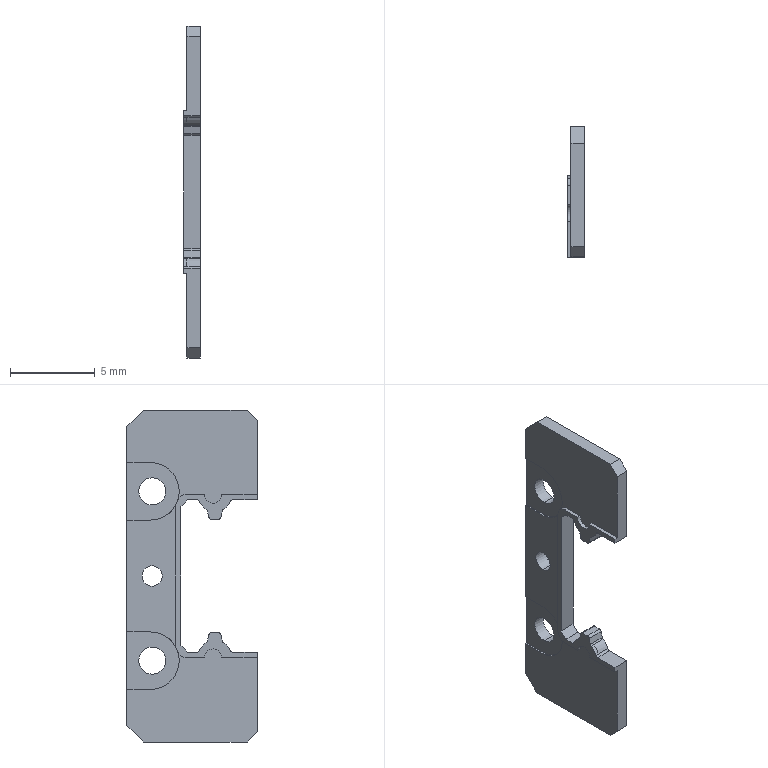Part | STEP file | EndSeal_MGN9 | 1 solid | 71 faces | box 1 x 7.7 x 19.6 mm | volume 85.449 mm3 | plane 38 | cylinder 33 | commonest cylinder face diameters 0.3 x12 2 x8 1.2 x4 1.6 x4 1 x3 3.4 x2